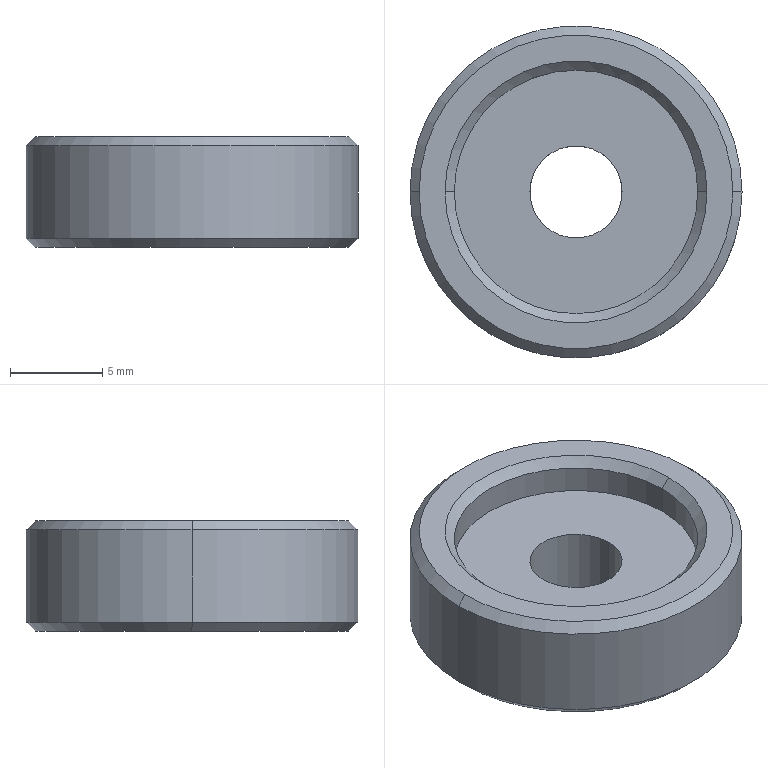Part | STEP file | 229H151428 Default | 1 solid | 15 faces | box 18 x 18 x 6 mm | volume 1155 mm3 | cone 6 | cylinder 6 | plane 3 | commonest cylinder face diameters 5 x2 13.2 x2 18 x2
STEP:
#1=CARTESIAN_POINT('',(-6.6,0.,5.5));
#2=VERTEX_POINT('',#1);
#3=CARTESIAN_POINT('',(6.6,0.,5.5));
#4=VERTEX_POINT('',#3);
#5=CARTESIAN_POINT('',(0.,0.,5.5));
#6=DIRECTION('',(0.,0.,1.));
#7=DIRECTION('',(1.,0.,0.));
#8=AXIS2_PLACEMENT_3D('',#5,#6,#7);
#9=CIRCLE('',#8,6.6);
#10=EDGE_CURVE('',#2,#4,#9,.T.);
#11=ORIENTED_EDGE('',*,*,#10,.F.);
#12=CARTESIAN_POINT('',(-7.1,0.,6.));
#13=VERTEX_POINT('',#12);
#14=CARTESIAN_POINT('',(-6.6,0.,5.5));
#15=DIRECTION('',(-0.7071,0.,0.7071));
#16=VECTOR('',#15,1000.);
#17=LINE('',#14,#16);
#18=EDGE_CURVE('',#2,#13,#17,.T.);
#19=ORIENTED_EDGE('',*,*,#18,.T.);
#20=CARTESIAN_POINT('',(7.1,0.,6.));
#21=VERTEX_POINT('',#20);
#22=CARTESIAN_POINT('',(0.,0.,6.));
#23=DIRECTION('',(0.,0.,-1.));
#24=DIRECTION('',(1.,0.,0.));
#25=AXIS2_PLACEMENT_3D('',#22,#23,#24);
#26=CIRCLE('',#25,7.1);
#27=EDGE_CURVE('',#21,#13,#26,.T.);
#28=ORIENTED_EDGE('',*,*,#27,.F.);
#29=CARTESIAN_POINT('',(6.6,0.,5.5));
#30=DIRECTION('',(0.7071,0.,0.7071));
#31=VECTOR('',#30,1000.);
#32=LINE('',#29,#31);
#33=EDGE_CURVE('',#4,#21,#32,.T.);
#34=ORIENTED_EDGE('',*,*,#33,.F.);
#35=EDGE_LOOP('',(#11,#19,#28,#34));
#36=FACE_OUTER_BOUND('',#35,.T.);
#37=CARTESIAN_POINT('',(0.,0.,5.5));
#38=DIRECTION('',(0.,0.,1.));
#39=DIRECTION('',(1.,0.,0.));
#40=AXIS2_PLACEMENT_3D('',#37,#38,#39);
#41=CONICAL_SURFACE('',#40,6.6,0.7854);
#42=ADVANCED_FACE('',(#36),#41,.F.);
#43=CARTESIAN_POINT('',(-8.5,0.,0.));
#44=VERTEX_POINT('',#43);
#45=CARTESIAN_POINT('',(8.5,0.,0.));
#46=VERTEX_POINT('',#45);
#47=CARTESIAN_POINT('',(0.,0.,0.));
#48=DIRECTION('',(0.,0.,-1.));
#49=DIRECTION('',(1.,0.,0.));
#50=AXIS2_PLACEMENT_3D('',#47,#48,#49);
#51=CIRCLE('',#50,8.5);
#52=EDGE_CURVE('',#44,#46,#51,.T.);
#53=ORIENTED_EDGE('',*,*,#52,.F.);
#54=CARTESIAN_POINT('',(-9.,0.,0.5));
#55=VERTEX_POINT('',#54);
#56=CARTESIAN_POINT('',(-9.,0.,0.5));
#57=DIRECTION('',(-0.7071,0.,0.7071));
#58=VECTOR('',#57,1000.);
#59=LINE('',#56,#58);
#60=EDGE_CURVE('',#44,#55,#59,.T.);
#61=ORIENTED_EDGE('',*,*,#60,.T.);
#62=CARTESIAN_POINT('',(9.,0.,0.5));
#63=VERTEX_POINT('',#62);
#64=CARTESIAN_POINT('',(0.,0.,0.5));
#65=DIRECTION('',(0.,0.,1.));
#66=DIRECTION('',(1.,0.,0.));
#67=AXIS2_PLACEMENT_3D('',#64,#65,#66);
#68=CIRCLE('',#67,9.);
#69=EDGE_CURVE('',#63,#55,#68,.T.);
#70=ORIENTED_EDGE('',*,*,#69,.F.);
#71=CARTESIAN_POINT('',(9.,0.,0.5));
#72=DIRECTION('',(0.7071,0.,0.7071));
#73=VECTOR('',#72,1000.);
#74=LINE('',#71,#73);
#75=EDGE_CURVE('',#46,#63,#74,.T.);
#76=ORIENTED_EDGE('',*,*,#75,.F.);
#77=EDGE_LOOP('',(#53,#61,#70,#76));
#78=FACE_OUTER_BOUND('',#77,.T.);
#79=CARTESIAN_POINT('',(0.,0.,0.5));
#80=DIRECTION('',(0.,0.,1.));
#81=DIRECTION('',(1.,0.,0.));
#82=AXIS2_PLACEMENT_3D('',#79,#80,#81);
#83=CONICAL_SURFACE('',#82,9.,0.7854);
#84=ADVANCED_FACE('',(#78),#83,.T.);
#85=CARTESIAN_POINT('',(8.5,0.,6.));
#86=VERTEX_POINT('',#85);
#87=CARTESIAN_POINT('',(-8.5,0.,6.));
#88=VERTEX_POINT('',#87);
#89=CARTESIAN_POINT('',(0.,0.,6.));
#90=DIRECTION('',(0.,0.,1.));
#91=DIRECTION('',(1.,0.,0.));
#92=AXIS2_PLACEMENT_3D('',#89,#90,#91);
#93=CIRCLE('',#92,8.5);
#94=EDGE_CURVE('',#86,#88,#93,.T.);
#95=ORIENTED_EDGE('',*,*,#94,.F.);
#96=CARTESIAN_POINT('',(9.,0.,5.5));
#97=VERTEX_POINT('',#96);
#98=CARTESIAN_POINT('',(8.5,0.,6.));
#99=DIRECTION('',(0.7071,0.,-0.7071));
#100=VECTOR('',#99,1000.);
#101=LINE('',#98,#100);
#102=EDGE_CURVE('',#86,#97,#101,.T.);
#103=ORIENTED_EDGE('',*,*,#102,.T.);
#104=CARTESIAN_POINT('',(-9.,0.,5.5));
#105=VERTEX_POINT('',#104);
#106=CARTESIAN_POINT('',(0.,0.,5.5));
#107=DIRECTION('',(0.,0.,-1.));
#108=DIRECTION('',(1.,0.,0.));
#109=AXIS2_PLACEMENT_3D('',#106,#107,#108);
#110=CIRCLE('',#109,9.);
#111=EDGE_CURVE('',#105,#97,#110,.T.);
#112=ORIENTED_EDGE('',*,*,#111,.F.);
#113=CARTESIAN_POINT('',(-8.5,0.,6.));
#114=DIRECTION('',(-0.7071,0.,-0.7071));
#115=VECTOR('',#114,1000.);
#116=LINE('',#113,#115);
#117=EDGE_CURVE('',#88,#105,#116,.T.);
#118=ORIENTED_EDGE('',*,*,#117,.F.);
#119=EDGE_LOOP('',(#95,#103,#112,#118));
#120=FACE_OUTER_BOUND('',#119,.T.);
#121=CARTESIAN_POINT('',(0.,0.,6.));
#122=DIRECTION('',(0.,0.,-1.));
#123=DIRECTION('',(-1.,0.,0.));
#124=AXIS2_PLACEMENT_3D('',#121,#122,#123);
#125=CONICAL_SURFACE('',#124,8.5,0.7854);
#126=ADVANCED_FACE('',(#120),#125,.T.);
#127=CARTESIAN_POINT('',(-2.5,0.,4.));
#128=VERTEX_POINT('',#127);
#129=CARTESIAN_POINT('',(2.5,0.,4.));
#130=VERTEX_POINT('',#129);
#131=CARTESIAN_POINT('',(0.,0.,4.));
#132=DIRECTION('',(0.,0.,1.));
#133=DIRECTION('',(1.,0.,0.));
#134=AXIS2_PLACEMENT_3D('',#131,#132,#133);
#135=CIRCLE('',#134,2.5);
#136=EDGE_CURVE('',#128,#130,#135,.T.);
#137=ORIENTED_EDGE('',*,*,#136,.T.);
#138=CARTESIAN_POINT('',(2.5,0.,0.));
#139=VERTEX_POINT('',#138);
#140=CARTESIAN_POINT('',(2.5,0.,0.));
#141=DIRECTION('',(0.,0.,-1.));
#142=VECTOR('',#141,1000.);
#143=LINE('',#140,#142);
#144=EDGE_CURVE('',#130,#139,#143,.T.);
#145=ORIENTED_EDGE('',*,*,#144,.T.);
#146=CARTESIAN_POINT('',(-2.5,0.,0.));
#147=VERTEX_POINT('',#146);
#148=CARTESIAN_POINT('',(0.,0.,0.));
#149=DIRECTION('',(0.,0.,-1.));
#150=DIRECTION('',(-1.,0.,0.));
#151=AXIS2_PLACEMENT_3D('',#148,#149,#150);
#152=CIRCLE('',#151,2.5);
#153=EDGE_CURVE('',#139,#147,#152,.T.);
#154=ORIENTED_EDGE('',*,*,#153,.T.);
#155=CARTESIAN_POINT('',(-2.5,0.,0.));
#156=DIRECTION('',(0.,0.,-1.));
#157=VECTOR('',#156,1000.);
#158=LINE('',#155,#157);
#159=EDGE_CURVE('',#128,#147,#158,.T.);
#160=ORIENTED_EDGE('',*,*,#159,.F.);
#161=EDGE_LOOP('',(#137,#145,#154,#160));
#162=FACE_OUTER_BOUND('',#161,.T.);
#163=CARTESIAN_POINT('',(0.,0.,0.));
#164=DIRECTION('',(0.,0.,-1.));
#165=DIRECTION('',(-1.,0.,0.));
#166=AXIS2_PLACEMENT_3D('',#163,#164,#165);
#167=CYLINDRICAL_SURFACE('',#166,2.5);
#168=ADVANCED_FACE('',(#162),#167,.F.);
#169=CARTESIAN_POINT('',(-6.6,0.,4.));
#170=VERTEX_POINT('',#169);
#171=CARTESIAN_POINT('',(6.6,0.,4.));
#172=VERTEX_POINT('',#171);
#173=CARTESIAN_POINT('',(0.,0.,4.));
#174=DIRECTION('',(0.,0.,1.));
#175=DIRECTION('',(1.,0.,0.));
#176=AXIS2_PLACEMENT_3D('',#173,#174,#175);
#177=CIRCLE('',#176,6.6);
#178=EDGE_CURVE('',#170,#172,#177,.T.);
#179=ORIENTED_EDGE('',*,*,#178,.F.);
#180=CARTESIAN_POINT('',(-6.6,0.,4.));
#181=DIRECTION('',(0.,0.,1.));
#182=VECTOR('',#181,1000.);
#183=LINE('',#180,#182);
#184=EDGE_CURVE('',#170,#2,#183,.T.);
#185=ORIENTED_EDGE('',*,*,#184,.T.);
#186=ORIENTED_EDGE('',*,*,#10,.T.);
#187=CARTESIAN_POINT('',(6.6,0.,4.));
#188=DIRECTION('',(0.,0.,1.));
#189=VECTOR('',#188,1000.);
#190=LINE('',#187,#189);
#191=EDGE_CURVE('',#172,#4,#190,.T.);
#192=ORIENTED_EDGE('',*,*,#191,.F.);
#193=EDGE_LOOP('',(#179,#185,#186,#192));
#194=FACE_OUTER_BOUND('',#193,.T.);
#195=CARTESIAN_POINT('',(0.,0.,4.));
#196=DIRECTION('',(0.,0.,1.));
#197=DIRECTION('',(1.,0.,0.));
#198=AXIS2_PLACEMENT_3D('',#195,#196,#197);
#199=CYLINDRICAL_SURFACE('',#198,6.6);
#200=ADVANCED_FACE('',(#194),#199,.F.);
#201=ORIENTED_EDGE('',*,*,#111,.T.);
#202=CARTESIAN_POINT('',(9.,0.,6.));
#203=DIRECTION('',(0.,0.,-1.));
#204=VECTOR('',#203,1000.);
#205=LINE('',#202,#204);
#206=EDGE_CURVE('',#97,#63,#205,.T.);
#207=ORIENTED_EDGE('',*,*,#206,.T.);
#208=ORIENTED_EDGE('',*,*,#69,.T.);
#209=CARTESIAN_POINT('',(-9.,0.,6.));
#210=DIRECTION('',(0.,0.,-1.));
#211=VECTOR('',#210,1000.);
#212=LINE('',#209,#211);
#213=EDGE_CURVE('',#105,#55,#212,.T.);
#214=ORIENTED_EDGE('',*,*,#213,.F.);
#215=EDGE_LOOP('',(#201,#207,#208,#214));
#216=FACE_OUTER_BOUND('',#215,.T.);
#217=CARTESIAN_POINT('',(0.,0.,6.));
#218=DIRECTION('',(0.,0.,-1.));
#219=DIRECTION('',(-1.,0.,0.));
#220=AXIS2_PLACEMENT_3D('',#217,#218,#219);
#221=CYLINDRICAL_SURFACE('',#220,9.);
#222=ADVANCED_FACE('',(#216),#221,.T.);
#223=ORIENTED_EDGE('',*,*,#206,.F.);
#224=CARTESIAN_POINT('',(0.,0.,5.5));
#225=DIRECTION('',(0.,0.,-1.));
#226=DIRECTION('',(1.,0.,0.));
#227=AXIS2_PLACEMENT_3D('',#224,#225,#226);
#228=CIRCLE('',#227,9.);
#229=EDGE_CURVE('',#97,#105,#228,.T.);
#230=ORIENTED_EDGE('',*,*,#229,.T.);
#231=ORIENTED_EDGE('',*,*,#213,.T.);
#232=CARTESIAN_POINT('',(0.,0.,0.5));
#233=DIRECTION('',(0.,0.,1.));
#234=DIRECTION('',(1.,0.,0.));
#235=AXIS2_PLACEMENT_3D('',#232,#233,#234);
#236=CIRCLE('',#235,9.);
#237=EDGE_CURVE('',#55,#63,#236,.T.);
#238=ORIENTED_EDGE('',*,*,#237,.T.);
#239=EDGE_LOOP('',(#223,#230,#231,#238));
#240=FACE_OUTER_BOUND('',#239,.T.);
#241=CARTESIAN_POINT('',(0.,0.,6.));
#242=DIRECTION('',(0.,0.,-1.));
#243=DIRECTION('',(-1.,0.,0.));
#244=AXIS2_PLACEMENT_3D('',#241,#242,#243);
#245=CYLINDRICAL_SURFACE('',#244,9.);
#246=ADVANCED_FACE('',(#240),#245,.T.);
#247=ORIENTED_EDGE('',*,*,#27,.T.);
#248=CARTESIAN_POINT('',(0.,0.,6.));
#249=DIRECTION('',(0.,0.,-1.));
#250=DIRECTION('',(1.,0.,0.));
#251=AXIS2_PLACEMENT_3D('',#248,#249,#250);
#252=CIRCLE('',#251,7.1);
#253=EDGE_CURVE('',#13,#21,#252,.T.);
#254=ORIENTED_EDGE('',*,*,#253,.T.);
#255=EDGE_LOOP('',(#247,#254));
#256=FACE_BOUND('',#255,.T.);
#257=CARTESIAN_POINT('',(0.,0.,6.));
#258=DIRECTION('',(0.,0.,1.));
#259=DIRECTION('',(1.,0.,0.));
#260=AXIS2_PLACEMENT_3D('',#257,#258,#259);
#261=CIRCLE('',#260,8.5);
#262=EDGE_CURVE('',#88,#86,#261,.T.);
#263=ORIENTED_EDGE('',*,*,#262,.T.);
#264=ORIENTED_EDGE('',*,*,#94,.T.);
#265=EDGE_LOOP('',(#263,#264));
#266=FACE_OUTER_BOUND('',#265,.T.);
#267=CARTESIAN_POINT('',(0.,0.,6.));
#268=DIRECTION('',(0.,0.,1.));
#269=DIRECTION('',(1.,0.,0.));
#270=AXIS2_PLACEMENT_3D('',#267,#268,#269);
#271=PLANE('',#270);
#272=ADVANCED_FACE('',(#256,#266),#271,.T.);
#273=CARTESIAN_POINT('',(0.,0.,0.));
#274=DIRECTION('',(0.,0.,-1.));
#275=DIRECTION('',(1.,0.,0.));
#276=AXIS2_PLACEMENT_3D('',#273,#274,#275);
#277=CIRCLE('',#276,8.5);
#278=EDGE_CURVE('',#46,#44,#277,.T.);
#279=ORIENTED_EDGE('',*,*,#278,.T.);
#280=ORIENTED_EDGE('',*,*,#52,.T.);
#281=EDGE_LOOP('',(#279,#280));
#282=FACE_OUTER_BOUND('',#281,.T.);
#283=CARTESIAN_POINT('',(0.,0.,0.));
#284=DIRECTION('',(0.,0.,-1.));
#285=DIRECTION('',(-1.,0.,0.));
#286=AXIS2_PLACEMENT_3D('',#283,#284,#285);
#287=CIRCLE('',#286,2.5);
#288=EDGE_CURVE('',#147,#139,#287,.T.);
#289=ORIENTED_EDGE('',*,*,#288,.F.);
#290=ORIENTED_EDGE('',*,*,#153,.F.);
#291=EDGE_LOOP('',(#289,#290));
#292=FACE_BOUND('',#291,.T.);
#293=CARTESIAN_POINT('',(0.,0.,0.));
#294=DIRECTION('',(0.,0.,1.));
#295=DIRECTION('',(1.,0.,0.));
#296=AXIS2_PLACEMENT_3D('',#293,#294,#295);
#297=PLANE('',#296);
#298=ADVANCED_FACE('',(#282,#292),#297,.F.);
#299=ORIENTED_EDGE('',*,*,#184,.F.);
#300=CARTESIAN_POINT('',(0.,0.,4.));
#301=DIRECTION('',(0.,0.,1.));
#302=DIRECTION('',(1.,0.,0.));
#303=AXIS2_PLACEMENT_3D('',#300,#301,#302);
#304=CIRCLE('',#303,6.6);
#305=EDGE_CURVE('',#172,#170,#304,.T.);
#306=ORIENTED_EDGE('',*,*,#305,.F.);
#307=ORIENTED_EDGE('',*,*,#191,.T.);
#308=CARTESIAN_POINT('',(0.,0.,5.5));
#309=DIRECTION('',(0.,0.,1.));
#310=DIRECTION('',(1.,0.,0.));
#311=AXIS2_PLACEMENT_3D('',#308,#309,#310);
#312=CIRCLE('',#311,6.6);
#313=EDGE_CURVE('',#4,#2,#312,.T.);
#314=ORIENTED_EDGE('',*,*,#313,.T.);
#315=EDGE_LOOP('',(#299,#306,#307,#314));
#316=FACE_OUTER_BOUND('',#315,.T.);
#317=CARTESIAN_POINT('',(0.,0.,4.));
#318=DIRECTION('',(0.,0.,1.));
#319=DIRECTION('',(1.,0.,0.));
#320=AXIS2_PLACEMENT_3D('',#317,#318,#319);
#321=CYLINDRICAL_SURFACE('',#320,6.6);
#322=ADVANCED_FACE('',(#316),#321,.F.);
#323=ORIENTED_EDGE('',*,*,#136,.F.);
#324=CARTESIAN_POINT('',(0.,0.,4.));
#325=DIRECTION('',(0.,0.,1.));
#326=DIRECTION('',(1.,0.,0.));
#327=AXIS2_PLACEMENT_3D('',#324,#325,#326);
#328=CIRCLE('',#327,2.5);
#329=EDGE_CURVE('',#130,#128,#328,.T.);
#330=ORIENTED_EDGE('',*,*,#329,.F.);
#331=EDGE_LOOP('',(#323,#330));
#332=FACE_BOUND('',#331,.T.);
#333=ORIENTED_EDGE('',*,*,#305,.T.);
#334=ORIENTED_EDGE('',*,*,#178,.T.);
#335=EDGE_LOOP('',(#333,#334));
#336=FACE_OUTER_BOUND('',#335,.T.);
#337=CARTESIAN_POINT('',(0.,0.,4.));
#338=DIRECTION('',(0.,0.,1.));
#339=DIRECTION('',(1.,0.,0.));
#340=AXIS2_PLACEMENT_3D('',#337,#338,#339);
#341=PLANE('',#340);
#342=ADVANCED_FACE('',(#332,#336),#341,.T.);
#343=ORIENTED_EDGE('',*,*,#144,.F.);
#344=ORIENTED_EDGE('',*,*,#329,.T.);
#345=ORIENTED_EDGE('',*,*,#159,.T.);
#346=ORIENTED_EDGE('',*,*,#288,.T.);
#347=EDGE_LOOP('',(#343,#344,#345,#346));
#348=FACE_OUTER_BOUND('',#347,.T.);
#349=CARTESIAN_POINT('',(0.,0.,0.));
#350=DIRECTION('',(0.,0.,-1.));
#351=DIRECTION('',(-1.,0.,0.));
#352=AXIS2_PLACEMENT_3D('',#349,#350,#351);
#353=CYLINDRICAL_SURFACE('',#352,2.5);
#354=ADVANCED_FACE('',(#348),#353,.F.);
#355=ORIENTED_EDGE('',*,*,#102,.F.);
#356=ORIENTED_EDGE('',*,*,#262,.F.);
#357=ORIENTED_EDGE('',*,*,#117,.T.);
#358=ORIENTED_EDGE('',*,*,#229,.F.);
#359=EDGE_LOOP('',(#355,#356,#357,#358));
#360=FACE_OUTER_BOUND('',#359,.T.);
#361=CARTESIAN_POINT('',(0.,0.,6.));
#362=DIRECTION('',(0.,0.,-1.));
#363=DIRECTION('',(-1.,0.,0.));
#364=AXIS2_PLACEMENT_3D('',#361,#362,#363);
#365=CONICAL_SURFACE('',#364,8.5,0.7854);
#366=ADVANCED_FACE('',(#360),#365,.T.);
#367=ORIENTED_EDGE('',*,*,#60,.F.);
#368=ORIENTED_EDGE('',*,*,#278,.F.);
#369=ORIENTED_EDGE('',*,*,#75,.T.);
#370=ORIENTED_EDGE('',*,*,#237,.F.);
#371=EDGE_LOOP('',(#367,#368,#369,#370));
#372=FACE_OUTER_BOUND('',#371,.T.);
#373=CARTESIAN_POINT('',(0.,0.,0.5));
#374=DIRECTION('',(0.,0.,1.));
#375=DIRECTION('',(1.,0.,0.));
#376=AXIS2_PLACEMENT_3D('',#373,#374,#375);
#377=CONICAL_SURFACE('',#376,9.,0.7854);
#378=ADVANCED_FACE('',(#372),#377,.T.);
#379=ORIENTED_EDGE('',*,*,#18,.F.);
#380=ORIENTED_EDGE('',*,*,#313,.F.);
#381=ORIENTED_EDGE('',*,*,#33,.T.);
#382=ORIENTED_EDGE('',*,*,#253,.F.);
#383=EDGE_LOOP('',(#379,#380,#381,#382));
#384=FACE_OUTER_BOUND('',#383,.T.);
#385=CARTESIAN_POINT('',(0.,0.,5.5));
#386=DIRECTION('',(0.,0.,1.));
#387=DIRECTION('',(1.,0.,0.));
#388=AXIS2_PLACEMENT_3D('',#385,#386,#387);
#389=CONICAL_SURFACE('',#388,6.6,0.7854);
#390=ADVANCED_FACE('',(#384),#389,.F.);
#391=CLOSED_SHELL('',(#42,#84,#126,#168,#200,#222,#246,#272,#298,#322,#342,#354,#366,#378,#390));
#392=MANIFOLD_SOLID_BREP('',#391);
#393=CARTESIAN_POINT('',(0.,0.,0.));
#394=DIRECTION('',(0.,0.,1.));
#395=DIRECTION('',(1.,0.,0.));
#396=AXIS2_PLACEMENT_3D('',#393,#394,#395);
#397=(LENGTH_UNIT()NAMED_UNIT(*)SI_UNIT(.MILLI.,.METRE.));
#398=UNCERTAINTY_MEASURE_WITH_UNIT(LENGTH_MEASURE(0.00001),#397,'','');
#399=(NAMED_UNIT(*)PLANE_ANGLE_UNIT()SI_UNIT($,.RADIAN.));
#400=(NAMED_UNIT(*)SI_UNIT($,.STERADIAN.)SOLID_ANGLE_UNIT());
#401=(GEOMETRIC_REPRESENTATION_CONTEXT(3)GLOBAL_UNCERTAINTY_ASSIGNED_CONTEXT((#398))GLOBAL_UNIT_ASSIGNED_CONTEXT((#397,#399,#400))REPRESENTATION_CONTEXT('',''));
#402=ADVANCED_BREP_SHAPE_REPRESENTATION('',(#392,#396),#401);